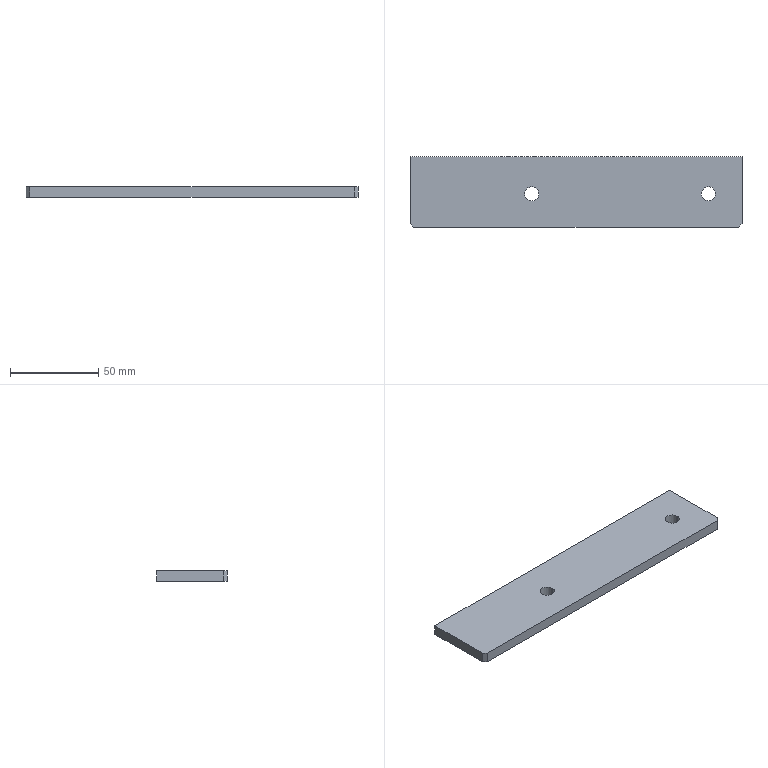Part | SolidWorks | features Chamfer 1, Extrusion 1, ICE 1 | 1 solid | 12 faces | box 188 x 40 x 6 mm | volume 44493 mm3 | plane 8 | cylinder 4 | commonest cylinder face diameters 8 x4
STEP:
#1=CARTESIAN_POINT('',(-29.,-1.,0.));
#2=VERTEX_POINT('',#1);
#3=CARTESIAN_POINT('',(-21.,-1.,0.));
#4=VERTEX_POINT('',#3);
#5=CARTESIAN_POINT('',(-25.,-1.,0.));
#6=DIRECTION('',(0.,0.,1.));
#7=DIRECTION('',(1.,0.,0.));
#8=AXIS2_PLACEMENT_3D('',#5,#6,#7);
#9=CIRCLE('',#8,4.);
#10=EDGE_CURVE('',#2,#4,#9,.T.);
#11=ORIENTED_EDGE('',*,*,#10,.F.);
#12=CARTESIAN_POINT('',(-29.,-1.,6.));
#13=VERTEX_POINT('',#12);
#14=CARTESIAN_POINT('',(-29.,-1.,0.));
#15=DIRECTION('',(0.,0.,1.));
#16=VECTOR('',#15,1000.);
#17=LINE('',#14,#16);
#18=EDGE_CURVE('',#2,#13,#17,.T.);
#19=ORIENTED_EDGE('',*,*,#18,.T.);
#20=CARTESIAN_POINT('',(-21.,-1.,6.));
#21=VERTEX_POINT('',#20);
#22=CARTESIAN_POINT('',(-25.,-1.,6.));
#23=DIRECTION('',(0.,0.,1.));
#24=DIRECTION('',(1.,0.,0.));
#25=AXIS2_PLACEMENT_3D('',#22,#23,#24);
#26=CIRCLE('',#25,4.);
#27=EDGE_CURVE('',#13,#21,#26,.T.);
#28=ORIENTED_EDGE('',*,*,#27,.T.);
#29=CARTESIAN_POINT('',(-21.,-1.,0.));
#30=DIRECTION('',(0.,0.,1.));
#31=VECTOR('',#30,1000.);
#32=LINE('',#29,#31);
#33=EDGE_CURVE('',#4,#21,#32,.T.);
#34=ORIENTED_EDGE('',*,*,#33,.F.);
#35=EDGE_LOOP('',(#11,#19,#28,#34));
#36=FACE_OUTER_BOUND('',#35,.T.);
#37=CARTESIAN_POINT('',(-25.,-1.,0.));
#38=DIRECTION('',(0.,0.,1.));
#39=DIRECTION('',(1.,0.,0.));
#40=AXIS2_PLACEMENT_3D('',#37,#38,#39);
#41=CYLINDRICAL_SURFACE('',#40,4.);
#42=ADVANCED_FACE('',(#36),#41,.F.);
#43=CARTESIAN_POINT('',(71.,-1.,0.));
#44=VERTEX_POINT('',#43);
#45=CARTESIAN_POINT('',(79.,-1.,0.));
#46=VERTEX_POINT('',#45);
#47=CARTESIAN_POINT('',(75.,-1.,0.));
#48=DIRECTION('',(0.,0.,1.));
#49=DIRECTION('',(1.,0.,0.));
#50=AXIS2_PLACEMENT_3D('',#47,#48,#49);
#51=CIRCLE('',#50,4.);
#52=EDGE_CURVE('',#44,#46,#51,.T.);
#53=ORIENTED_EDGE('',*,*,#52,.F.);
#54=CARTESIAN_POINT('',(71.,-1.,6.));
#55=VERTEX_POINT('',#54);
#56=CARTESIAN_POINT('',(71.,-1.,0.));
#57=DIRECTION('',(0.,0.,1.));
#58=VECTOR('',#57,1000.);
#59=LINE('',#56,#58);
#60=EDGE_CURVE('',#44,#55,#59,.T.);
#61=ORIENTED_EDGE('',*,*,#60,.T.);
#62=CARTESIAN_POINT('',(79.,-1.,6.));
#63=VERTEX_POINT('',#62);
#64=CARTESIAN_POINT('',(75.,-1.,6.));
#65=DIRECTION('',(0.,0.,1.));
#66=DIRECTION('',(1.,0.,0.));
#67=AXIS2_PLACEMENT_3D('',#64,#65,#66);
#68=CIRCLE('',#67,4.);
#69=EDGE_CURVE('',#55,#63,#68,.T.);
#70=ORIENTED_EDGE('',*,*,#69,.T.);
#71=CARTESIAN_POINT('',(79.,-1.,0.));
#72=DIRECTION('',(0.,0.,1.));
#73=VECTOR('',#72,1000.);
#74=LINE('',#71,#73);
#75=EDGE_CURVE('',#46,#63,#74,.T.);
#76=ORIENTED_EDGE('',*,*,#75,.F.);
#77=EDGE_LOOP('',(#53,#61,#70,#76));
#78=FACE_OUTER_BOUND('',#77,.T.);
#79=CARTESIAN_POINT('',(75.,-1.,0.));
#80=DIRECTION('',(0.,0.,1.));
#81=DIRECTION('',(1.,0.,0.));
#82=AXIS2_PLACEMENT_3D('',#79,#80,#81);
#83=CYLINDRICAL_SURFACE('',#82,4.);
#84=ADVANCED_FACE('',(#78),#83,.F.);
#85=CARTESIAN_POINT('',(-94.,20.,0.));
#86=VERTEX_POINT('',#85);
#87=CARTESIAN_POINT('',(-94.,-18.,0.));
#88=VERTEX_POINT('',#87);
#89=CARTESIAN_POINT('',(-94.,20.,0.));
#90=DIRECTION('',(0.,-1.,0.));
#91=VECTOR('',#90,1000.);
#92=LINE('',#89,#91);
#93=EDGE_CURVE('',#86,#88,#92,.T.);
#94=ORIENTED_EDGE('',*,*,#93,.T.);
#95=CARTESIAN_POINT('',(-94.,-18.,6.));
#96=VERTEX_POINT('',#95);
#97=CARTESIAN_POINT('',(-94.,-18.,6.));
#98=DIRECTION('',(0.,0.,1.));
#99=VECTOR('',#98,1000.);
#100=LINE('',#97,#99);
#101=EDGE_CURVE('',#88,#96,#100,.T.);
#102=ORIENTED_EDGE('',*,*,#101,.T.);
#103=CARTESIAN_POINT('',(-94.,20.,6.));
#104=VERTEX_POINT('',#103);
#105=CARTESIAN_POINT('',(-94.,20.,6.));
#106=DIRECTION('',(0.,-1.,0.));
#107=VECTOR('',#106,1000.);
#108=LINE('',#105,#107);
#109=EDGE_CURVE('',#104,#96,#108,.T.);
#110=ORIENTED_EDGE('',*,*,#109,.F.);
#111=CARTESIAN_POINT('',(-94.,20.,6.));
#112=DIRECTION('',(0.,0.,-1.));
#113=VECTOR('',#112,1000.);
#114=LINE('',#111,#113);
#115=EDGE_CURVE('',#104,#86,#114,.T.);
#116=ORIENTED_EDGE('',*,*,#115,.T.);
#117=EDGE_LOOP('',(#94,#102,#110,#116));
#118=FACE_OUTER_BOUND('',#117,.T.);
#119=CARTESIAN_POINT('',(-94.,20.,6.));
#120=DIRECTION('',(1.,0.,0.));
#121=DIRECTION('',(0.,1.,0.));
#122=AXIS2_PLACEMENT_3D('',#119,#120,#121);
#123=PLANE('',#122);
#124=ADVANCED_FACE('',(#118),#123,.F.);
#125=CARTESIAN_POINT('',(-92.,-20.,0.));
#126=VERTEX_POINT('',#125);
#127=CARTESIAN_POINT('',(92.,-20.,0.));
#128=VERTEX_POINT('',#127);
#129=CARTESIAN_POINT('',(94.,-20.,0.));
#130=DIRECTION('',(1.,0.,0.));
#131=VECTOR('',#130,1000.);
#132=LINE('',#129,#131);
#133=EDGE_CURVE('',#126,#128,#132,.T.);
#134=ORIENTED_EDGE('',*,*,#133,.T.);
#135=CARTESIAN_POINT('',(92.,-20.,6.));
#136=VERTEX_POINT('',#135);
#137=CARTESIAN_POINT('',(92.,-20.,6.));
#138=DIRECTION('',(0.,0.,1.));
#139=VECTOR('',#138,1000.);
#140=LINE('',#137,#139);
#141=EDGE_CURVE('',#128,#136,#140,.T.);
#142=ORIENTED_EDGE('',*,*,#141,.T.);
#143=CARTESIAN_POINT('',(-92.,-20.,6.));
#144=VERTEX_POINT('',#143);
#145=CARTESIAN_POINT('',(94.,-20.,6.));
#146=DIRECTION('',(1.,0.,0.));
#147=VECTOR('',#146,1000.);
#148=LINE('',#145,#147);
#149=EDGE_CURVE('',#144,#136,#148,.T.);
#150=ORIENTED_EDGE('',*,*,#149,.F.);
#151=CARTESIAN_POINT('',(-92.,-20.,6.));
#152=DIRECTION('',(0.,0.,-1.));
#153=VECTOR('',#152,1000.);
#154=LINE('',#151,#153);
#155=EDGE_CURVE('',#144,#126,#154,.T.);
#156=ORIENTED_EDGE('',*,*,#155,.T.);
#157=EDGE_LOOP('',(#134,#142,#150,#156));
#158=FACE_OUTER_BOUND('',#157,.T.);
#159=CARTESIAN_POINT('',(94.,-20.,6.));
#160=DIRECTION('',(0.,1.,0.));
#161=DIRECTION('',(-1.,0.,0.));
#162=AXIS2_PLACEMENT_3D('',#159,#160,#161);
#163=PLANE('',#162);
#164=ADVANCED_FACE('',(#158),#163,.F.);
#165=CARTESIAN_POINT('',(94.,-18.,6.));
#166=VERTEX_POINT('',#165);
#167=CARTESIAN_POINT('',(94.,20.,6.));
#168=VERTEX_POINT('',#167);
#169=CARTESIAN_POINT('',(94.,20.,6.));
#170=DIRECTION('',(0.,1.,0.));
#171=VECTOR('',#170,1000.);
#172=LINE('',#169,#171);
#173=EDGE_CURVE('',#166,#168,#172,.T.);
#174=ORIENTED_EDGE('',*,*,#173,.F.);
#175=CARTESIAN_POINT('',(94.,-18.,0.));
#176=VERTEX_POINT('',#175);
#177=CARTESIAN_POINT('',(94.,-18.,6.));
#178=DIRECTION('',(0.,0.,-1.));
#179=VECTOR('',#178,1000.);
#180=LINE('',#177,#179);
#181=EDGE_CURVE('',#166,#176,#180,.T.);
#182=ORIENTED_EDGE('',*,*,#181,.T.);
#183=CARTESIAN_POINT('',(94.,20.,0.));
#184=VERTEX_POINT('',#183);
#185=CARTESIAN_POINT('',(94.,20.,0.));
#186=DIRECTION('',(0.,1.,0.));
#187=VECTOR('',#186,1000.);
#188=LINE('',#185,#187);
#189=EDGE_CURVE('',#176,#184,#188,.T.);
#190=ORIENTED_EDGE('',*,*,#189,.T.);
#191=CARTESIAN_POINT('',(94.,20.,6.));
#192=DIRECTION('',(0.,0.,-1.));
#193=VECTOR('',#192,1000.);
#194=LINE('',#191,#193);
#195=EDGE_CURVE('',#168,#184,#194,.T.);
#196=ORIENTED_EDGE('',*,*,#195,.F.);
#197=EDGE_LOOP('',(#174,#182,#190,#196));
#198=FACE_OUTER_BOUND('',#197,.T.);
#199=CARTESIAN_POINT('',(94.,20.,6.));
#200=DIRECTION('',(-1.,0.,0.));
#201=DIRECTION('',(0.,0.,1.));
#202=AXIS2_PLACEMENT_3D('',#199,#200,#201);
#203=PLANE('',#202);
#204=ADVANCED_FACE('',(#198),#203,.F.);
#205=CARTESIAN_POINT('',(94.,20.,0.));
#206=DIRECTION('',(-1.,0.,0.));
#207=VECTOR('',#206,1000.);
#208=LINE('',#205,#207);
#209=EDGE_CURVE('',#184,#86,#208,.T.);
#210=ORIENTED_EDGE('',*,*,#209,.T.);
#211=ORIENTED_EDGE('',*,*,#115,.F.);
#212=CARTESIAN_POINT('',(94.,20.,6.));
#213=DIRECTION('',(-1.,0.,0.));
#214=VECTOR('',#213,1000.);
#215=LINE('',#212,#214);
#216=EDGE_CURVE('',#168,#104,#215,.T.);
#217=ORIENTED_EDGE('',*,*,#216,.F.);
#218=ORIENTED_EDGE('',*,*,#195,.T.);
#219=EDGE_LOOP('',(#210,#211,#217,#218));
#220=FACE_OUTER_BOUND('',#219,.T.);
#221=CARTESIAN_POINT('',(94.,20.,6.));
#222=DIRECTION('',(0.,-1.,0.));
#223=DIRECTION('',(1.,0.,0.));
#224=AXIS2_PLACEMENT_3D('',#221,#222,#223);
#225=PLANE('',#224);
#226=ADVANCED_FACE('',(#220),#225,.F.);
#227=CARTESIAN_POINT('',(-25.,-1.,6.));
#228=DIRECTION('',(0.,0.,1.));
#229=DIRECTION('',(1.,0.,0.));
#230=AXIS2_PLACEMENT_3D('',#227,#228,#229);
#231=CIRCLE('',#230,4.);
#232=EDGE_CURVE('',#21,#13,#231,.T.);
#233=ORIENTED_EDGE('',*,*,#232,.F.);
#234=ORIENTED_EDGE('',*,*,#27,.F.);
#235=EDGE_LOOP('',(#233,#234));
#236=FACE_BOUND('',#235,.T.);
#237=CARTESIAN_POINT('',(75.,-1.,6.));
#238=DIRECTION('',(0.,0.,1.));
#239=DIRECTION('',(1.,0.,0.));
#240=AXIS2_PLACEMENT_3D('',#237,#238,#239);
#241=CIRCLE('',#240,4.);
#242=EDGE_CURVE('',#63,#55,#241,.T.);
#243=ORIENTED_EDGE('',*,*,#242,.F.);
#244=ORIENTED_EDGE('',*,*,#69,.F.);
#245=EDGE_LOOP('',(#243,#244));
#246=FACE_BOUND('',#245,.T.);
#247=ORIENTED_EDGE('',*,*,#149,.T.);
#248=CARTESIAN_POINT('',(94.,-18.,6.));
#249=DIRECTION('',(0.7071,0.7071,0.));
#250=VECTOR('',#249,1000.);
#251=LINE('',#248,#250);
#252=EDGE_CURVE('',#136,#166,#251,.T.);
#253=ORIENTED_EDGE('',*,*,#252,.T.);
#254=ORIENTED_EDGE('',*,*,#173,.T.);
#255=ORIENTED_EDGE('',*,*,#216,.T.);
#256=ORIENTED_EDGE('',*,*,#109,.T.);
#257=CARTESIAN_POINT('',(-92.,-20.,6.));
#258=DIRECTION('',(0.7071,-0.7071,0.));
#259=VECTOR('',#258,1000.);
#260=LINE('',#257,#259);
#261=EDGE_CURVE('',#96,#144,#260,.T.);
#262=ORIENTED_EDGE('',*,*,#261,.T.);
#263=EDGE_LOOP('',(#247,#253,#254,#255,#256,#262));
#264=FACE_OUTER_BOUND('',#263,.T.);
#265=CARTESIAN_POINT('',(0.,0.,6.));
#266=DIRECTION('',(0.,0.,-1.));
#267=DIRECTION('',(-1.,0.,0.));
#268=AXIS2_PLACEMENT_3D('',#265,#266,#267);
#269=PLANE('',#268);
#270=ADVANCED_FACE('',(#236,#246,#264),#269,.F.);
#271=CARTESIAN_POINT('',(-25.,-1.,0.));
#272=DIRECTION('',(0.,0.,1.));
#273=DIRECTION('',(1.,0.,0.));
#274=AXIS2_PLACEMENT_3D('',#271,#272,#273);
#275=CIRCLE('',#274,4.);
#276=EDGE_CURVE('',#4,#2,#275,.T.);
#277=ORIENTED_EDGE('',*,*,#276,.T.);
#278=ORIENTED_EDGE('',*,*,#10,.T.);
#279=EDGE_LOOP('',(#277,#278));
#280=FACE_BOUND('',#279,.T.);
#281=CARTESIAN_POINT('',(75.,-1.,0.));
#282=DIRECTION('',(0.,0.,1.));
#283=DIRECTION('',(1.,0.,0.));
#284=AXIS2_PLACEMENT_3D('',#281,#282,#283);
#285=CIRCLE('',#284,4.);
#286=EDGE_CURVE('',#46,#44,#285,.T.);
#287=ORIENTED_EDGE('',*,*,#286,.T.);
#288=ORIENTED_EDGE('',*,*,#52,.T.);
#289=EDGE_LOOP('',(#287,#288));
#290=FACE_BOUND('',#289,.T.);
#291=ORIENTED_EDGE('',*,*,#189,.F.);
#292=CARTESIAN_POINT('',(56.,-56.,0.));
#293=DIRECTION('',(-0.7071,-0.7071,0.));
#294=VECTOR('',#293,1000.);
#295=LINE('',#292,#294);
#296=EDGE_CURVE('',#176,#128,#295,.T.);
#297=ORIENTED_EDGE('',*,*,#296,.T.);
#298=ORIENTED_EDGE('',*,*,#133,.F.);
#299=CARTESIAN_POINT('',(-56.,-56.,0.));
#300=DIRECTION('',(-0.7071,0.7071,0.));
#301=VECTOR('',#300,1000.);
#302=LINE('',#299,#301);
#303=EDGE_CURVE('',#126,#88,#302,.T.);
#304=ORIENTED_EDGE('',*,*,#303,.T.);
#305=ORIENTED_EDGE('',*,*,#93,.F.);
#306=ORIENTED_EDGE('',*,*,#209,.F.);
#307=EDGE_LOOP('',(#291,#297,#298,#304,#305,#306));
#308=FACE_OUTER_BOUND('',#307,.T.);
#309=CARTESIAN_POINT('',(0.,0.,0.));
#310=DIRECTION('',(0.,0.,-1.));
#311=DIRECTION('',(-1.,0.,0.));
#312=AXIS2_PLACEMENT_3D('',#309,#310,#311);
#313=PLANE('',#312);
#314=ADVANCED_FACE('',(#280,#290,#308),#313,.T.);
#315=ORIENTED_EDGE('',*,*,#60,.F.);
#316=ORIENTED_EDGE('',*,*,#286,.F.);
#317=ORIENTED_EDGE('',*,*,#75,.T.);
#318=ORIENTED_EDGE('',*,*,#242,.T.);
#319=EDGE_LOOP('',(#315,#316,#317,#318));
#320=FACE_OUTER_BOUND('',#319,.T.);
#321=CARTESIAN_POINT('',(75.,-1.,0.));
#322=DIRECTION('',(0.,0.,1.));
#323=DIRECTION('',(1.,0.,0.));
#324=AXIS2_PLACEMENT_3D('',#321,#322,#323);
#325=CYLINDRICAL_SURFACE('',#324,4.);
#326=ADVANCED_FACE('',(#320),#325,.F.);
#327=ORIENTED_EDGE('',*,*,#18,.F.);
#328=ORIENTED_EDGE('',*,*,#276,.F.);
#329=ORIENTED_EDGE('',*,*,#33,.T.);
#330=ORIENTED_EDGE('',*,*,#232,.T.);
#331=EDGE_LOOP('',(#327,#328,#329,#330));
#332=FACE_OUTER_BOUND('',#331,.T.);
#333=CARTESIAN_POINT('',(-25.,-1.,0.));
#334=DIRECTION('',(0.,0.,1.));
#335=DIRECTION('',(1.,0.,0.));
#336=AXIS2_PLACEMENT_3D('',#333,#334,#335);
#337=CYLINDRICAL_SURFACE('',#336,4.);
#338=ADVANCED_FACE('',(#332),#337,.F.);
#339=ORIENTED_EDGE('',*,*,#252,.F.);
#340=ORIENTED_EDGE('',*,*,#141,.F.);
#341=ORIENTED_EDGE('',*,*,#296,.F.);
#342=ORIENTED_EDGE('',*,*,#181,.F.);
#343=EDGE_LOOP('',(#339,#340,#341,#342));
#344=FACE_OUTER_BOUND('',#343,.T.);
#345=CARTESIAN_POINT('',(94.,-18.,6.));
#346=DIRECTION('',(-0.7071,0.7071,0.));
#347=DIRECTION('',(0.,0.,-1.));
#348=AXIS2_PLACEMENT_3D('',#345,#346,#347);
#349=PLANE('',#348);
#350=ADVANCED_FACE('',(#344),#349,.F.);
#351=ORIENTED_EDGE('',*,*,#261,.F.);
#352=ORIENTED_EDGE('',*,*,#101,.F.);
#353=ORIENTED_EDGE('',*,*,#303,.F.);
#354=ORIENTED_EDGE('',*,*,#155,.F.);
#355=EDGE_LOOP('',(#351,#352,#353,#354));
#356=FACE_OUTER_BOUND('',#355,.T.);
#357=CARTESIAN_POINT('',(-92.,-20.,6.));
#358=DIRECTION('',(0.7071,0.7071,0.));
#359=DIRECTION('',(0.,0.,-1.));
#360=AXIS2_PLACEMENT_3D('',#357,#358,#359);
#361=PLANE('',#360);
#362=ADVANCED_FACE('',(#356),#361,.F.);
#363=CLOSED_SHELL('',(#42,#84,#124,#164,#204,#226,#270,#314,#326,#338,#350,#362));
#364=MANIFOLD_SOLID_BREP('',#363);
#365=CARTESIAN_POINT('',(0.,0.,0.));
#366=DIRECTION('',(0.,0.,1.));
#367=DIRECTION('',(1.,0.,0.));
#368=AXIS2_PLACEMENT_3D('',#365,#366,#367);
#369=(LENGTH_UNIT()NAMED_UNIT(*)SI_UNIT(.MILLI.,.METRE.));
#370=UNCERTAINTY_MEASURE_WITH_UNIT(LENGTH_MEASURE(0.00001),#369,'','');
#371=(NAMED_UNIT(*)PLANE_ANGLE_UNIT()SI_UNIT($,.RADIAN.));
#372=(NAMED_UNIT(*)SI_UNIT($,.STERADIAN.)SOLID_ANGLE_UNIT());
#373=(GEOMETRIC_REPRESENTATION_CONTEXT(3)GLOBAL_UNCERTAINTY_ASSIGNED_CONTEXT((#370))GLOBAL_UNIT_ASSIGNED_CONTEXT((#369,#371,#372))REPRESENTATION_CONTEXT('',''));
#374=ADVANCED_BREP_SHAPE_REPRESENTATION('',(#364,#368),#373);